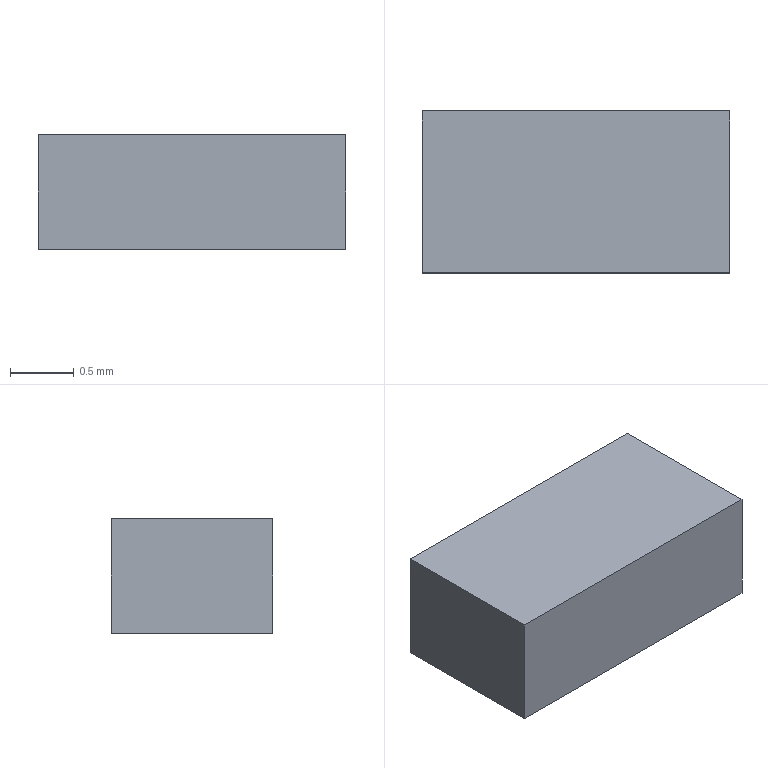Part | Creo | 1 solid | 6 faces | box 2.413 x 1.27 x 0.9 mm | volume 2.758 mm3 | plane 6
STEP:
#1=CARTESIAN_POINT('',(0.,0.,0.));
#2=DIRECTION('',(0.,0.,1.));
#3=DIRECTION('',(1.,0.,0.));
#4=AXIS2_PLACEMENT_3D('',#1,#2,#3);
#5=CARTESIAN_POINT('',(-1.206,0.635,0.));
#6=VERTEX_POINT('',#5);
#7=CARTESIAN_POINT('',(-1.206,-0.635,0.));
#8=VERTEX_POINT('',#7);
#9=CARTESIAN_POINT('',(-1.206,0.635,0.));
#10=DIRECTION('',(0.,-1.,0.));
#11=VECTOR('',#10,1.27);
#12=LINE('',#9,#11);
#13=EDGE_CURVE('',#6,#8,#12,.T.);
#14=ORIENTED_EDGE('',*,*,#13,.T.);
#15=CARTESIAN_POINT('',(1.206,-0.635,0.));
#16=VERTEX_POINT('',#15);
#17=CARTESIAN_POINT('',(-1.206,-0.635,0.));
#18=DIRECTION('',(1.,0.,0.));
#19=VECTOR('',#18,2.413);
#20=LINE('',#17,#19);
#21=EDGE_CURVE('',#8,#16,#20,.T.);
#22=ORIENTED_EDGE('',*,*,#21,.T.);
#23=CARTESIAN_POINT('',(1.206,0.635,0.));
#24=VERTEX_POINT('',#23);
#25=CARTESIAN_POINT('',(1.206,-0.635,0.));
#26=DIRECTION('',(0.,1.,0.));
#27=VECTOR('',#26,1.27);
#28=LINE('',#25,#27);
#29=EDGE_CURVE('',#16,#24,#28,.T.);
#30=ORIENTED_EDGE('',*,*,#29,.T.);
#31=CARTESIAN_POINT('',(1.206,0.635,0.));
#32=DIRECTION('',(-1.,0.,0.));
#33=VECTOR('',#32,2.413);
#34=LINE('',#31,#33);
#35=EDGE_CURVE('',#24,#6,#34,.T.);
#36=ORIENTED_EDGE('',*,*,#35,.T.);
#37=EDGE_LOOP('',(#14,#22,#30,#36));
#38=FACE_OUTER_BOUND('',#37,.F.);
#39=CARTESIAN_POINT('',(0.,0.,0.));
#40=DIRECTION('',(0.,0.,1.));
#41=DIRECTION('',(1.,0.,0.));
#42=AXIS2_PLACEMENT_3D('',#39,#40,#41);
#43=PLANE('',#42);
#44=ADVANCED_FACE('',(#38),#43,.F.);
#45=ORIENTED_EDGE('',*,*,#13,.F.);
#46=CARTESIAN_POINT('',(-1.206,0.635,0.9));
#47=VERTEX_POINT('',#46);
#48=CARTESIAN_POINT('',(-1.206,0.635,0.));
#49=DIRECTION('',(0.,0.,1.));
#50=VECTOR('',#49,0.9);
#51=LINE('',#48,#50);
#52=EDGE_CURVE('',#6,#47,#51,.T.);
#53=ORIENTED_EDGE('',*,*,#52,.T.);
#54=CARTESIAN_POINT('',(-1.206,-0.635,0.9));
#55=VERTEX_POINT('',#54);
#56=CARTESIAN_POINT('',(-1.206,0.635,0.9));
#57=DIRECTION('',(0.,-1.,0.));
#58=VECTOR('',#57,1.27);
#59=LINE('',#56,#58);
#60=EDGE_CURVE('',#47,#55,#59,.T.);
#61=ORIENTED_EDGE('',*,*,#60,.T.);
#62=CARTESIAN_POINT('',(-1.206,-0.635,0.));
#63=DIRECTION('',(0.,0.,1.));
#64=VECTOR('',#63,0.9);
#65=LINE('',#62,#64);
#66=EDGE_CURVE('',#8,#55,#65,.T.);
#67=ORIENTED_EDGE('',*,*,#66,.F.);
#68=EDGE_LOOP('',(#45,#53,#61,#67));
#69=FACE_OUTER_BOUND('',#68,.F.);
#70=CARTESIAN_POINT('',(-1.206,0.635,0.));
#71=DIRECTION('',(-1.,0.,0.));
#72=DIRECTION('',(0.,-1.,0.));
#73=AXIS2_PLACEMENT_3D('',#70,#71,#72);
#74=PLANE('',#73);
#75=ADVANCED_FACE('',(#69),#74,.T.);
#76=ORIENTED_EDGE('',*,*,#35,.F.);
#77=CARTESIAN_POINT('',(1.206,0.635,0.9));
#78=VERTEX_POINT('',#77);
#79=CARTESIAN_POINT('',(1.206,0.635,0.));
#80=DIRECTION('',(0.,0.,1.));
#81=VECTOR('',#80,0.9);
#82=LINE('',#79,#81);
#83=EDGE_CURVE('',#24,#78,#82,.T.);
#84=ORIENTED_EDGE('',*,*,#83,.T.);
#85=CARTESIAN_POINT('',(1.206,0.635,0.9));
#86=DIRECTION('',(-1.,0.,0.));
#87=VECTOR('',#86,2.413);
#88=LINE('',#85,#87);
#89=EDGE_CURVE('',#78,#47,#88,.T.);
#90=ORIENTED_EDGE('',*,*,#89,.T.);
#91=ORIENTED_EDGE('',*,*,#52,.F.);
#92=EDGE_LOOP('',(#76,#84,#90,#91));
#93=FACE_OUTER_BOUND('',#92,.F.);
#94=CARTESIAN_POINT('',(1.206,0.635,0.));
#95=DIRECTION('',(0.,1.,0.));
#96=DIRECTION('',(-1.,0.,0.));
#97=AXIS2_PLACEMENT_3D('',#94,#95,#96);
#98=PLANE('',#97);
#99=ADVANCED_FACE('',(#93),#98,.T.);
#100=ORIENTED_EDGE('',*,*,#29,.F.);
#101=CARTESIAN_POINT('',(1.206,-0.635,0.9));
#102=VERTEX_POINT('',#101);
#103=CARTESIAN_POINT('',(1.206,-0.635,0.));
#104=DIRECTION('',(0.,0.,1.));
#105=VECTOR('',#104,0.9);
#106=LINE('',#103,#105);
#107=EDGE_CURVE('',#16,#102,#106,.T.);
#108=ORIENTED_EDGE('',*,*,#107,.T.);
#109=CARTESIAN_POINT('',(1.206,-0.635,0.9));
#110=DIRECTION('',(0.,1.,0.));
#111=VECTOR('',#110,1.27);
#112=LINE('',#109,#111);
#113=EDGE_CURVE('',#102,#78,#112,.T.);
#114=ORIENTED_EDGE('',*,*,#113,.T.);
#115=ORIENTED_EDGE('',*,*,#83,.F.);
#116=EDGE_LOOP('',(#100,#108,#114,#115));
#117=FACE_OUTER_BOUND('',#116,.F.);
#118=CARTESIAN_POINT('',(1.206,-0.635,0.));
#119=DIRECTION('',(1.,0.,0.));
#120=DIRECTION('',(0.,1.,0.));
#121=AXIS2_PLACEMENT_3D('',#118,#119,#120);
#122=PLANE('',#121);
#123=ADVANCED_FACE('',(#117),#122,.T.);
#124=ORIENTED_EDGE('',*,*,#21,.F.);
#125=ORIENTED_EDGE('',*,*,#66,.T.);
#126=CARTESIAN_POINT('',(-1.206,-0.635,0.9));
#127=DIRECTION('',(1.,0.,0.));
#128=VECTOR('',#127,2.413);
#129=LINE('',#126,#128);
#130=EDGE_CURVE('',#55,#102,#129,.T.);
#131=ORIENTED_EDGE('',*,*,#130,.T.);
#132=ORIENTED_EDGE('',*,*,#107,.F.);
#133=EDGE_LOOP('',(#124,#125,#131,#132));
#134=FACE_OUTER_BOUND('',#133,.F.);
#135=CARTESIAN_POINT('',(-1.206,-0.635,0.));
#136=DIRECTION('',(0.,-1.,0.));
#137=DIRECTION('',(1.,0.,0.));
#138=AXIS2_PLACEMENT_3D('',#135,#136,#137);
#139=PLANE('',#138);
#140=ADVANCED_FACE('',(#134),#139,.T.);
#141=ORIENTED_EDGE('',*,*,#60,.F.);
#142=ORIENTED_EDGE('',*,*,#89,.F.);
#143=ORIENTED_EDGE('',*,*,#113,.F.);
#144=ORIENTED_EDGE('',*,*,#130,.F.);
#145=EDGE_LOOP('',(#141,#142,#143,#144));
#146=FACE_OUTER_BOUND('',#145,.F.);
#147=CARTESIAN_POINT('',(0.,0.,0.9));
#148=DIRECTION('',(0.,0.,1.));
#149=DIRECTION('',(1.,0.,0.));
#150=AXIS2_PLACEMENT_3D('',#147,#148,#149);
#151=PLANE('',#150);
#152=ADVANCED_FACE('',(#146),#151,.T.);
#153=CLOSED_SHELL('',(#44,#75,#99,#123,#140,#152));
#154=MANIFOLD_SOLID_BREP('',#153);
#155=(LENGTH_UNIT()NAMED_UNIT(*)SI_UNIT(.MILLI.,.METRE.));
#156=UNCERTAINTY_MEASURE_WITH_UNIT(LENGTH_MEASURE(0.0002871),#155,'','');
#157=(NAMED_UNIT(*)PLANE_ANGLE_UNIT()SI_UNIT($,.RADIAN.));
#158=PLANE_ANGLE_MEASURE_WITH_UNIT(PLANE_ANGLE_MEASURE(0.01745),#157);
#159=(CONVERSION_BASED_UNIT('DEGREE',#158)NAMED_UNIT(*)PLANE_ANGLE_UNIT());
#160=(NAMED_UNIT(*)SI_UNIT($,.STERADIAN.)SOLID_ANGLE_UNIT());
#161=(GEOMETRIC_REPRESENTATION_CONTEXT(3)GLOBAL_UNCERTAINTY_ASSIGNED_CONTEXT((#156))GLOBAL_UNIT_ASSIGNED_CONTEXT((#155,#159,#160))REPRESENTATION_CONTEXT('',''));
#162=ADVANCED_BREP_SHAPE_REPRESENTATION('',(#4,#154),#161);